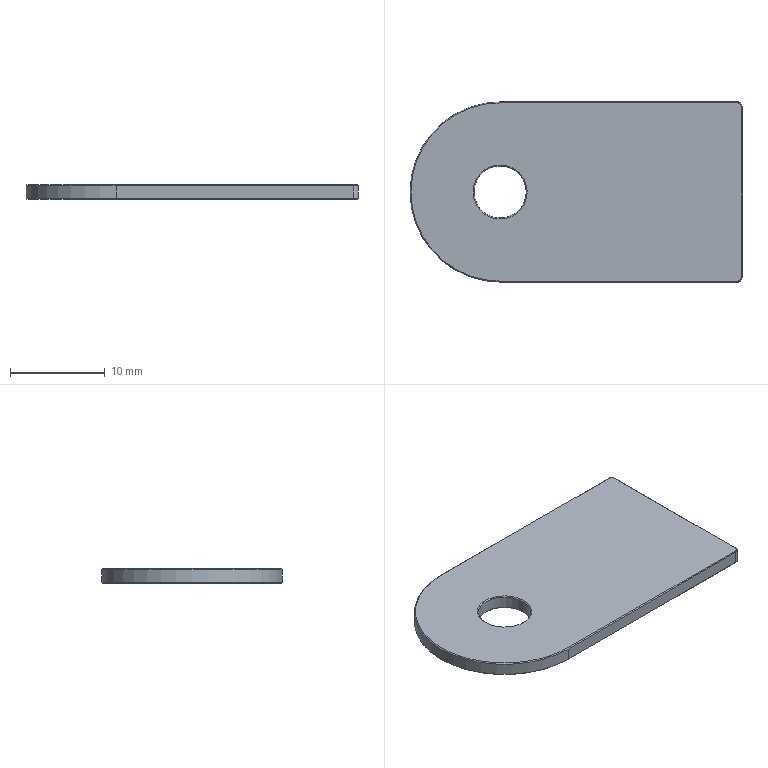Part | STEP file | SUPORTE PRENSA CABOS-A | 1 solid | 27 faces | box 35 x 19 x 1.5 mm | volume 902.431 mm3 | cone 11 | plane 11 | cylinder 5 | commonest cylinder face diameters 1 x2 5.5 x2 19 x1